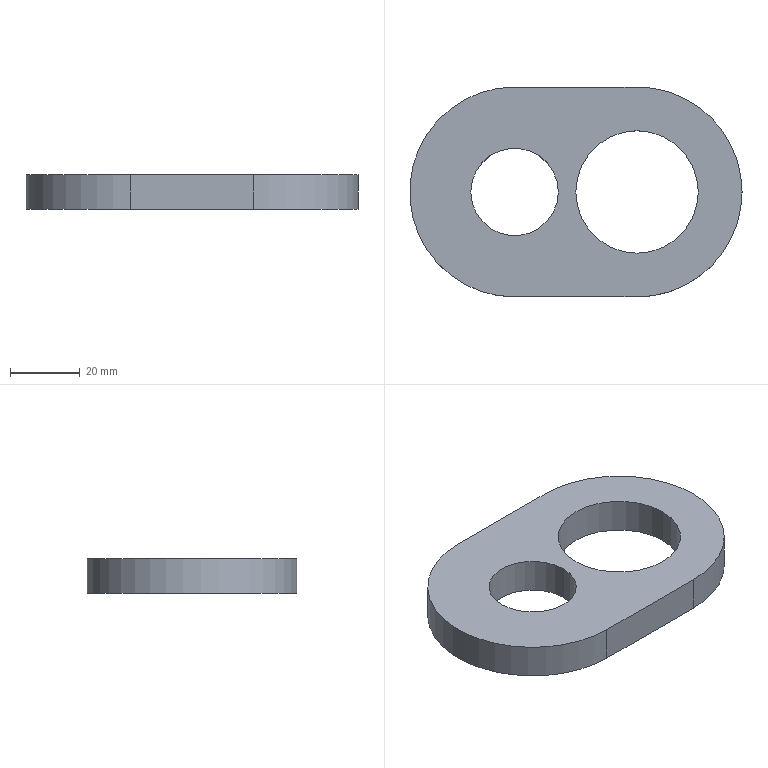Part | SolidWorks | features BaseBody 1 | 1 solid | 11 faces | box 95 x 60 x 10 mm | volume 34744 mm3 | cylinder 7 | plane 4 | commonest cylinder face diameters 60 x3 25 x2 35 x2
STEP:
#1=CARTESIAN_POINT('',(-30.,0.,0.));
#2=VERTEX_POINT('',#1);
#3=CARTESIAN_POINT('',(-5.,0.,0.));
#4=VERTEX_POINT('',#3);
#5=CARTESIAN_POINT('',(-17.5,0.,0.));
#6=DIRECTION('',(0.,0.,1.));
#7=DIRECTION('',(1.,0.,0.));
#8=AXIS2_PLACEMENT_3D('',#5,#6,#7);
#9=CIRCLE('',#8,12.5);
#10=EDGE_CURVE('',#2,#4,#9,.T.);
#11=ORIENTED_EDGE('',*,*,#10,.F.);
#12=CARTESIAN_POINT('',(-30.,0.,10.));
#13=VERTEX_POINT('',#12);
#14=CARTESIAN_POINT('',(-30.,0.,0.));
#15=DIRECTION('',(0.,0.,1.));
#16=VECTOR('',#15,1000.);
#17=LINE('',#14,#16);
#18=EDGE_CURVE('',#2,#13,#17,.T.);
#19=ORIENTED_EDGE('',*,*,#18,.T.);
#20=CARTESIAN_POINT('',(-5.,0.,10.));
#21=VERTEX_POINT('',#20);
#22=CARTESIAN_POINT('',(-17.5,0.,10.));
#23=DIRECTION('',(0.,0.,-1.));
#24=DIRECTION('',(1.,0.,0.));
#25=AXIS2_PLACEMENT_3D('',#22,#23,#24);
#26=CIRCLE('',#25,12.5);
#27=EDGE_CURVE('',#21,#13,#26,.T.);
#28=ORIENTED_EDGE('',*,*,#27,.F.);
#29=CARTESIAN_POINT('',(-5.,0.,0.));
#30=DIRECTION('',(0.,0.,1.));
#31=VECTOR('',#30,1000.);
#32=LINE('',#29,#31);
#33=EDGE_CURVE('',#4,#21,#32,.T.);
#34=ORIENTED_EDGE('',*,*,#33,.F.);
#35=EDGE_LOOP('',(#11,#19,#28,#34));
#36=FACE_OUTER_BOUND('',#35,.T.);
#37=CARTESIAN_POINT('',(-17.5,0.,0.));
#38=DIRECTION('',(0.,0.,1.));
#39=DIRECTION('',(1.,0.,0.));
#40=AXIS2_PLACEMENT_3D('',#37,#38,#39);
#41=CYLINDRICAL_SURFACE('',#40,12.5);
#42=ADVANCED_FACE('',(#36),#41,.F.);
#43=CARTESIAN_POINT('',(0.,0.,0.));
#44=VERTEX_POINT('',#43);
#45=CARTESIAN_POINT('',(35.,0.,0.));
#46=VERTEX_POINT('',#45);
#47=CARTESIAN_POINT('',(17.5,0.,0.));
#48=DIRECTION('',(0.,0.,1.));
#49=DIRECTION('',(1.,0.,0.));
#50=AXIS2_PLACEMENT_3D('',#47,#48,#49);
#51=CIRCLE('',#50,17.5);
#52=EDGE_CURVE('',#44,#46,#51,.T.);
#53=ORIENTED_EDGE('',*,*,#52,.F.);
#54=CARTESIAN_POINT('',(0.,0.,10.));
#55=VERTEX_POINT('',#54);
#56=CARTESIAN_POINT('',(0.,0.,0.));
#57=DIRECTION('',(0.,0.,1.));
#58=VECTOR('',#57,1000.);
#59=LINE('',#56,#58);
#60=EDGE_CURVE('',#44,#55,#59,.T.);
#61=ORIENTED_EDGE('',*,*,#60,.T.);
#62=CARTESIAN_POINT('',(35.,0.,10.));
#63=VERTEX_POINT('',#62);
#64=CARTESIAN_POINT('',(17.5,0.,10.));
#65=DIRECTION('',(0.,0.,-1.));
#66=DIRECTION('',(1.,0.,0.));
#67=AXIS2_PLACEMENT_3D('',#64,#65,#66);
#68=CIRCLE('',#67,17.5);
#69=EDGE_CURVE('',#63,#55,#68,.T.);
#70=ORIENTED_EDGE('',*,*,#69,.F.);
#71=CARTESIAN_POINT('',(35.,0.,0.));
#72=DIRECTION('',(0.,0.,1.));
#73=VECTOR('',#72,1000.);
#74=LINE('',#71,#73);
#75=EDGE_CURVE('',#46,#63,#74,.T.);
#76=ORIENTED_EDGE('',*,*,#75,.F.);
#77=EDGE_LOOP('',(#53,#61,#70,#76));
#78=FACE_OUTER_BOUND('',#77,.T.);
#79=CARTESIAN_POINT('',(17.5,0.,0.));
#80=DIRECTION('',(0.,0.,1.));
#81=DIRECTION('',(1.,0.,0.));
#82=AXIS2_PLACEMENT_3D('',#79,#80,#81);
#83=CYLINDRICAL_SURFACE('',#82,17.5);
#84=ADVANCED_FACE('',(#78),#83,.F.);
#85=CARTESIAN_POINT('',(17.5,-30.,0.));
#86=VERTEX_POINT('',#85);
#87=CARTESIAN_POINT('',(47.5,0.,0.));
#88=VERTEX_POINT('',#87);
#89=CARTESIAN_POINT('',(17.5,0.,0.));
#90=DIRECTION('',(0.,0.,1.));
#91=DIRECTION('',(1.,0.,0.));
#92=AXIS2_PLACEMENT_3D('',#89,#90,#91);
#93=CIRCLE('',#92,30.);
#94=EDGE_CURVE('',#86,#88,#93,.T.);
#95=ORIENTED_EDGE('',*,*,#94,.T.);
#96=CARTESIAN_POINT('',(47.5,0.,10.));
#97=VERTEX_POINT('',#96);
#98=CARTESIAN_POINT('',(47.5,0.,0.));
#99=DIRECTION('',(0.,0.,1.));
#100=VECTOR('',#99,1000.);
#101=LINE('',#98,#100);
#102=EDGE_CURVE('',#88,#97,#101,.T.);
#103=ORIENTED_EDGE('',*,*,#102,.T.);
#104=CARTESIAN_POINT('',(17.5,-30.,10.));
#105=VERTEX_POINT('',#104);
#106=CARTESIAN_POINT('',(17.5,0.,10.));
#107=DIRECTION('',(0.,0.,1.));
#108=DIRECTION('',(1.,0.,0.));
#109=AXIS2_PLACEMENT_3D('',#106,#107,#108);
#110=CIRCLE('',#109,30.);
#111=EDGE_CURVE('',#105,#97,#110,.T.);
#112=ORIENTED_EDGE('',*,*,#111,.F.);
#113=CARTESIAN_POINT('',(17.5,-30.,0.));
#114=DIRECTION('',(0.,0.,-1.));
#115=VECTOR('',#114,1000.);
#116=LINE('',#113,#115);
#117=EDGE_CURVE('',#105,#86,#116,.T.);
#118=ORIENTED_EDGE('',*,*,#117,.T.);
#119=EDGE_LOOP('',(#95,#103,#112,#118));
#120=FACE_OUTER_BOUND('',#119,.T.);
#121=CARTESIAN_POINT('',(17.5,0.,0.));
#122=DIRECTION('',(0.,0.,1.));
#123=DIRECTION('',(1.,0.,0.));
#124=AXIS2_PLACEMENT_3D('',#121,#122,#123);
#125=CYLINDRICAL_SURFACE('',#124,30.);
#126=ADVANCED_FACE('',(#120),#125,.T.);
#127=ORIENTED_EDGE('',*,*,#27,.T.);
#128=CARTESIAN_POINT('',(-17.5,0.,10.));
#129=DIRECTION('',(0.,0.,-1.));
#130=DIRECTION('',(1.,0.,0.));
#131=AXIS2_PLACEMENT_3D('',#128,#129,#130);
#132=CIRCLE('',#131,12.5);
#133=EDGE_CURVE('',#13,#21,#132,.T.);
#134=ORIENTED_EDGE('',*,*,#133,.T.);
#135=EDGE_LOOP('',(#127,#134));
#136=FACE_BOUND('',#135,.T.);
#137=ORIENTED_EDGE('',*,*,#69,.T.);
#138=CARTESIAN_POINT('',(17.5,0.,10.));
#139=DIRECTION('',(0.,0.,-1.));
#140=DIRECTION('',(1.,0.,0.));
#141=AXIS2_PLACEMENT_3D('',#138,#139,#140);
#142=CIRCLE('',#141,17.5);
#143=EDGE_CURVE('',#55,#63,#142,.T.);
#144=ORIENTED_EDGE('',*,*,#143,.T.);
#145=EDGE_LOOP('',(#137,#144));
#146=FACE_BOUND('',#145,.T.);
#147=ORIENTED_EDGE('',*,*,#111,.T.);
#148=CARTESIAN_POINT('',(17.5,30.,10.));
#149=VERTEX_POINT('',#148);
#150=CARTESIAN_POINT('',(17.5,0.,10.));
#151=DIRECTION('',(0.,0.,1.));
#152=DIRECTION('',(1.,0.,0.));
#153=AXIS2_PLACEMENT_3D('',#150,#151,#152);
#154=CIRCLE('',#153,30.);
#155=EDGE_CURVE('',#97,#149,#154,.T.);
#156=ORIENTED_EDGE('',*,*,#155,.T.);
#157=CARTESIAN_POINT('',(-17.5,30.,10.));
#158=VERTEX_POINT('',#157);
#159=CARTESIAN_POINT('',(0.,30.,10.));
#160=DIRECTION('',(-1.,0.,0.));
#161=VECTOR('',#160,1000.);
#162=LINE('',#159,#161);
#163=EDGE_CURVE('',#149,#158,#162,.T.);
#164=ORIENTED_EDGE('',*,*,#163,.T.);
#165=CARTESIAN_POINT('',(-17.5,-30.,10.));
#166=VERTEX_POINT('',#165);
#167=CARTESIAN_POINT('',(-17.5,0.,10.));
#168=DIRECTION('',(0.,0.,1.));
#169=DIRECTION('',(1.,0.,0.));
#170=AXIS2_PLACEMENT_3D('',#167,#168,#169);
#171=CIRCLE('',#170,30.);
#172=EDGE_CURVE('',#158,#166,#171,.T.);
#173=ORIENTED_EDGE('',*,*,#172,.T.);
#174=CARTESIAN_POINT('',(0.,-30.,10.));
#175=DIRECTION('',(1.,0.,0.));
#176=VECTOR('',#175,1000.);
#177=LINE('',#174,#176);
#178=EDGE_CURVE('',#166,#105,#177,.T.);
#179=ORIENTED_EDGE('',*,*,#178,.T.);
#180=EDGE_LOOP('',(#147,#156,#164,#173,#179));
#181=FACE_OUTER_BOUND('',#180,.T.);
#182=CARTESIAN_POINT('',(0.,0.,10.));
#183=DIRECTION('',(0.,0.,1.));
#184=DIRECTION('',(1.,0.,0.));
#185=AXIS2_PLACEMENT_3D('',#182,#183,#184);
#186=PLANE('',#185);
#187=ADVANCED_FACE('',(#136,#146,#181),#186,.T.);
#188=ORIENTED_EDGE('',*,*,#18,.F.);
#189=CARTESIAN_POINT('',(-17.5,0.,0.));
#190=DIRECTION('',(0.,0.,1.));
#191=DIRECTION('',(1.,0.,0.));
#192=AXIS2_PLACEMENT_3D('',#189,#190,#191);
#193=CIRCLE('',#192,12.5);
#194=EDGE_CURVE('',#4,#2,#193,.T.);
#195=ORIENTED_EDGE('',*,*,#194,.F.);
#196=ORIENTED_EDGE('',*,*,#33,.T.);
#197=ORIENTED_EDGE('',*,*,#133,.F.);
#198=EDGE_LOOP('',(#188,#195,#196,#197));
#199=FACE_OUTER_BOUND('',#198,.T.);
#200=CARTESIAN_POINT('',(-17.5,0.,0.));
#201=DIRECTION('',(0.,0.,1.));
#202=DIRECTION('',(1.,0.,0.));
#203=AXIS2_PLACEMENT_3D('',#200,#201,#202);
#204=CYLINDRICAL_SURFACE('',#203,12.5);
#205=ADVANCED_FACE('',(#199),#204,.F.);
#206=ORIENTED_EDGE('',*,*,#60,.F.);
#207=CARTESIAN_POINT('',(17.5,0.,0.));
#208=DIRECTION('',(0.,0.,1.));
#209=DIRECTION('',(1.,0.,0.));
#210=AXIS2_PLACEMENT_3D('',#207,#208,#209);
#211=CIRCLE('',#210,17.5);
#212=EDGE_CURVE('',#46,#44,#211,.T.);
#213=ORIENTED_EDGE('',*,*,#212,.F.);
#214=ORIENTED_EDGE('',*,*,#75,.T.);
#215=ORIENTED_EDGE('',*,*,#143,.F.);
#216=EDGE_LOOP('',(#206,#213,#214,#215));
#217=FACE_OUTER_BOUND('',#216,.T.);
#218=CARTESIAN_POINT('',(17.5,0.,0.));
#219=DIRECTION('',(0.,0.,1.));
#220=DIRECTION('',(1.,0.,0.));
#221=AXIS2_PLACEMENT_3D('',#218,#219,#220);
#222=CYLINDRICAL_SURFACE('',#221,17.5);
#223=ADVANCED_FACE('',(#217),#222,.F.);
#224=CARTESIAN_POINT('',(17.5,30.,0.));
#225=VERTEX_POINT('',#224);
#226=CARTESIAN_POINT('',(-17.5,30.,0.));
#227=VERTEX_POINT('',#226);
#228=CARTESIAN_POINT('',(-17.5,30.,0.));
#229=DIRECTION('',(-1.,0.,0.));
#230=VECTOR('',#229,1000.);
#231=LINE('',#228,#230);
#232=EDGE_CURVE('',#225,#227,#231,.T.);
#233=ORIENTED_EDGE('',*,*,#232,.T.);
#234=CARTESIAN_POINT('',(-17.5,30.,0.));
#235=DIRECTION('',(0.,0.,1.));
#236=VECTOR('',#235,1000.);
#237=LINE('',#234,#236);
#238=EDGE_CURVE('',#227,#158,#237,.T.);
#239=ORIENTED_EDGE('',*,*,#238,.T.);
#240=ORIENTED_EDGE('',*,*,#163,.F.);
#241=CARTESIAN_POINT('',(17.5,30.,0.));
#242=DIRECTION('',(0.,0.,-1.));
#243=VECTOR('',#242,1000.);
#244=LINE('',#241,#243);
#245=EDGE_CURVE('',#149,#225,#244,.T.);
#246=ORIENTED_EDGE('',*,*,#245,.T.);
#247=EDGE_LOOP('',(#233,#239,#240,#246));
#248=FACE_OUTER_BOUND('',#247,.T.);
#249=CARTESIAN_POINT('',(-17.5,30.,0.));
#250=DIRECTION('',(0.,1.,0.));
#251=DIRECTION('',(-1.,0.,0.));
#252=AXIS2_PLACEMENT_3D('',#249,#250,#251);
#253=PLANE('',#252);
#254=ADVANCED_FACE('',(#248),#253,.T.);
#255=ORIENTED_EDGE('',*,*,#102,.F.);
#256=CARTESIAN_POINT('',(17.5,0.,0.));
#257=DIRECTION('',(0.,0.,1.));
#258=DIRECTION('',(1.,0.,0.));
#259=AXIS2_PLACEMENT_3D('',#256,#257,#258);
#260=CIRCLE('',#259,30.);
#261=EDGE_CURVE('',#88,#225,#260,.T.);
#262=ORIENTED_EDGE('',*,*,#261,.T.);
#263=ORIENTED_EDGE('',*,*,#245,.F.);
#264=ORIENTED_EDGE('',*,*,#155,.F.);
#265=EDGE_LOOP('',(#255,#262,#263,#264));
#266=FACE_OUTER_BOUND('',#265,.T.);
#267=CARTESIAN_POINT('',(17.5,0.,0.));
#268=DIRECTION('',(0.,0.,1.));
#269=DIRECTION('',(1.,0.,0.));
#270=AXIS2_PLACEMENT_3D('',#267,#268,#269);
#271=CYLINDRICAL_SURFACE('',#270,30.);
#272=ADVANCED_FACE('',(#266),#271,.T.);
#273=CARTESIAN_POINT('',(-17.5,-30.,0.));
#274=VERTEX_POINT('',#273);
#275=CARTESIAN_POINT('',(17.5,-30.,0.));
#276=DIRECTION('',(1.,0.,0.));
#277=VECTOR('',#276,1000.);
#278=LINE('',#275,#277);
#279=EDGE_CURVE('',#274,#86,#278,.T.);
#280=ORIENTED_EDGE('',*,*,#279,.T.);
#281=ORIENTED_EDGE('',*,*,#117,.F.);
#282=ORIENTED_EDGE('',*,*,#178,.F.);
#283=CARTESIAN_POINT('',(-17.5,-30.,0.));
#284=DIRECTION('',(0.,0.,-1.));
#285=VECTOR('',#284,1000.);
#286=LINE('',#283,#285);
#287=EDGE_CURVE('',#166,#274,#286,.T.);
#288=ORIENTED_EDGE('',*,*,#287,.T.);
#289=EDGE_LOOP('',(#280,#281,#282,#288));
#290=FACE_OUTER_BOUND('',#289,.T.);
#291=CARTESIAN_POINT('',(17.5,-30.,0.));
#292=DIRECTION('',(0.,-1.,0.));
#293=DIRECTION('',(0.,0.,-1.));
#294=AXIS2_PLACEMENT_3D('',#291,#292,#293);
#295=PLANE('',#294);
#296=ADVANCED_FACE('',(#290),#295,.T.);
#297=CARTESIAN_POINT('',(-17.5,0.,0.));
#298=DIRECTION('',(0.,0.,1.));
#299=DIRECTION('',(1.,0.,0.));
#300=AXIS2_PLACEMENT_3D('',#297,#298,#299);
#301=CIRCLE('',#300,30.);
#302=EDGE_CURVE('',#227,#274,#301,.T.);
#303=ORIENTED_EDGE('',*,*,#302,.T.);
#304=ORIENTED_EDGE('',*,*,#287,.F.);
#305=ORIENTED_EDGE('',*,*,#172,.F.);
#306=ORIENTED_EDGE('',*,*,#238,.F.);
#307=EDGE_LOOP('',(#303,#304,#305,#306));
#308=FACE_OUTER_BOUND('',#307,.T.);
#309=CARTESIAN_POINT('',(-17.5,0.,0.));
#310=DIRECTION('',(0.,0.,1.));
#311=DIRECTION('',(1.,0.,0.));
#312=AXIS2_PLACEMENT_3D('',#309,#310,#311);
#313=CYLINDRICAL_SURFACE('',#312,30.);
#314=ADVANCED_FACE('',(#308),#313,.T.);
#315=ORIENTED_EDGE('',*,*,#194,.T.);
#316=ORIENTED_EDGE('',*,*,#10,.T.);
#317=EDGE_LOOP('',(#315,#316));
#318=FACE_BOUND('',#317,.T.);
#319=ORIENTED_EDGE('',*,*,#212,.T.);
#320=ORIENTED_EDGE('',*,*,#52,.T.);
#321=EDGE_LOOP('',(#319,#320));
#322=FACE_BOUND('',#321,.T.);
#323=ORIENTED_EDGE('',*,*,#302,.F.);
#324=ORIENTED_EDGE('',*,*,#232,.F.);
#325=ORIENTED_EDGE('',*,*,#261,.F.);
#326=ORIENTED_EDGE('',*,*,#94,.F.);
#327=ORIENTED_EDGE('',*,*,#279,.F.);
#328=EDGE_LOOP('',(#323,#324,#325,#326,#327));
#329=FACE_OUTER_BOUND('',#328,.T.);
#330=CARTESIAN_POINT('',(0.,0.,0.));
#331=DIRECTION('',(0.,0.,1.));
#332=DIRECTION('',(1.,0.,0.));
#333=AXIS2_PLACEMENT_3D('',#330,#331,#332);
#334=PLANE('',#333);
#335=ADVANCED_FACE('',(#318,#322,#329),#334,.F.);
#336=CLOSED_SHELL('',(#42,#84,#126,#187,#205,#223,#254,#272,#296,#314,#335));
#337=MANIFOLD_SOLID_BREP('',#336);
#338=CARTESIAN_POINT('',(0.,0.,0.));
#339=DIRECTION('',(0.,0.,1.));
#340=DIRECTION('',(1.,0.,0.));
#341=AXIS2_PLACEMENT_3D('',#338,#339,#340);
#342=(LENGTH_UNIT()NAMED_UNIT(*)SI_UNIT(.MILLI.,.METRE.));
#343=UNCERTAINTY_MEASURE_WITH_UNIT(LENGTH_MEASURE(0.00001),#342,'','');
#344=(NAMED_UNIT(*)PLANE_ANGLE_UNIT()SI_UNIT($,.RADIAN.));
#345=(NAMED_UNIT(*)SI_UNIT($,.STERADIAN.)SOLID_ANGLE_UNIT());
#346=(GEOMETRIC_REPRESENTATION_CONTEXT(3)GLOBAL_UNCERTAINTY_ASSIGNED_CONTEXT((#343))GLOBAL_UNIT_ASSIGNED_CONTEXT((#342,#344,#345))REPRESENTATION_CONTEXT('',''));
#347=ADVANCED_BREP_SHAPE_REPRESENTATION('',(#337,#341),#346);